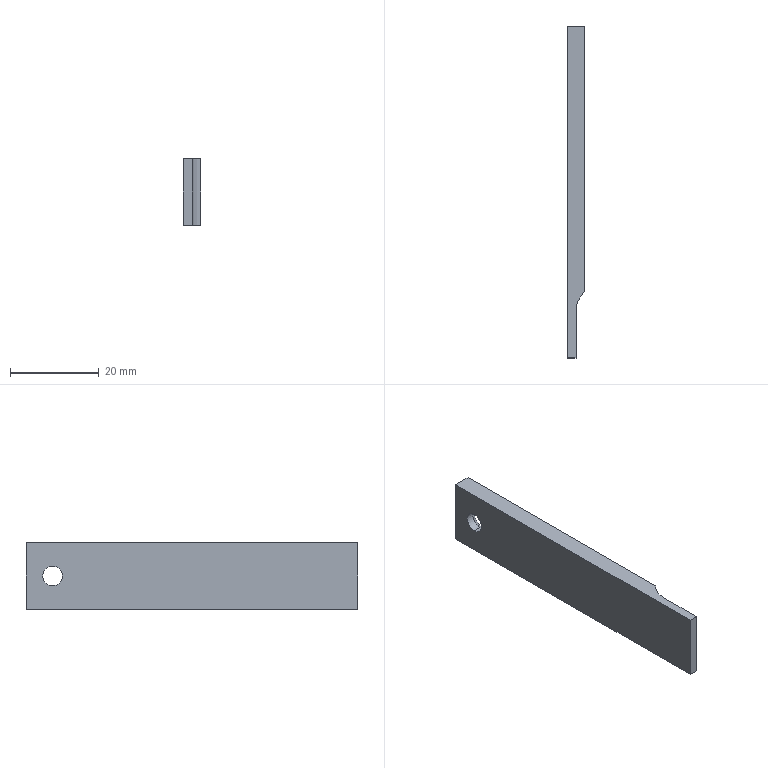Part | NX | features BREP 1 | 1 solid | 12 faces | box 4 x 75 x 15 mm | volume 3981 mm3 | plane 7 | cylinder 3 | cone 2 | commonest cylinder face diameters 4.5 x2 12 x1
STEP:
#1=CARTESIAN_POINT('',(-377.307,34.363,9.75));
#2=VERTEX_POINT('',#1);
#3=CARTESIAN_POINT('',(-377.307,34.363,5.25));
#4=VERTEX_POINT('',#3);
#5=CARTESIAN_POINT('',(-377.307,34.363,7.5));
#6=DIRECTION('',(1.,0.,0.));
#7=DIRECTION('',(0.,0.,-1.));
#8=AXIS2_PLACEMENT_3D('',#5,#6,#7);
#9=CIRCLE('',#8,2.25);
#10=EDGE_CURVE('',#2,#4,#9,.T.);
#11=ORIENTED_EDGE('',*,*,#10,.F.);
#12=CARTESIAN_POINT('',(-375.077,34.363,11.98));
#13=VERTEX_POINT('',#12);
#14=CARTESIAN_POINT('',(-375.077,34.363,11.98));
#15=DIRECTION('',(0.7071,0.,0.7071));
#16=VECTOR('',#15,1000.);
#17=LINE('',#14,#16);
#18=EDGE_CURVE('',#2,#13,#17,.T.);
#19=ORIENTED_EDGE('',*,*,#18,.T.);
#20=CARTESIAN_POINT('',(-375.077,34.363,3.02));
#21=VERTEX_POINT('',#20);
#22=CARTESIAN_POINT('',(-375.077,34.363,7.5));
#23=DIRECTION('',(1.,0.,0.));
#24=DIRECTION('',(0.,0.,-1.));
#25=AXIS2_PLACEMENT_3D('',#22,#23,#24);
#26=CIRCLE('',#25,4.48);
#27=EDGE_CURVE('',#13,#21,#26,.T.);
#28=ORIENTED_EDGE('',*,*,#27,.T.);
#29=CARTESIAN_POINT('',(-375.077,34.363,3.02));
#30=DIRECTION('',(0.7071,0.,-0.7071));
#31=VECTOR('',#30,1000.);
#32=LINE('',#29,#31);
#33=EDGE_CURVE('',#4,#21,#32,.T.);
#34=ORIENTED_EDGE('',*,*,#33,.F.);
#35=EDGE_LOOP('',(#11,#19,#28,#34));
#36=FACE_BOUND('',#35,.T.);
#37=CARTESIAN_POINT('',(-375.077,34.363,7.5));
#38=DIRECTION('',(1.,0.,0.));
#39=DIRECTION('',(0.,0.,-1.));
#40=AXIS2_PLACEMENT_3D('',#37,#38,#39);
#41=CONICAL_SURFACE('',#40,4.48,0.7854);
#42=ADVANCED_FACE('',(#36),#41,.F.);
#43=CARTESIAN_POINT('',(-379.077,34.363,9.75));
#44=VERTEX_POINT('',#43);
#45=CARTESIAN_POINT('',(-379.077,34.363,5.25));
#46=VERTEX_POINT('',#45);
#47=CARTESIAN_POINT('',(-379.077,34.363,7.5));
#48=DIRECTION('',(1.,0.,0.));
#49=DIRECTION('',(0.,0.,-1.));
#50=AXIS2_PLACEMENT_3D('',#47,#48,#49);
#51=CIRCLE('',#50,2.25);
#52=EDGE_CURVE('',#44,#46,#51,.T.);
#53=ORIENTED_EDGE('',*,*,#52,.F.);
#54=CARTESIAN_POINT('',(-375.077,34.363,9.75));
#55=DIRECTION('',(1.,0.,0.));
#56=VECTOR('',#55,1000.);
#57=LINE('',#54,#56);
#58=EDGE_CURVE('',#44,#2,#57,.T.);
#59=ORIENTED_EDGE('',*,*,#58,.T.);
#60=ORIENTED_EDGE('',*,*,#10,.T.);
#61=CARTESIAN_POINT('',(-375.077,34.363,5.25));
#62=DIRECTION('',(1.,0.,0.));
#63=VECTOR('',#62,1000.);
#64=LINE('',#61,#63);
#65=EDGE_CURVE('',#46,#4,#64,.T.);
#66=ORIENTED_EDGE('',*,*,#65,.F.);
#67=EDGE_LOOP('',(#53,#59,#60,#66));
#68=FACE_BOUND('',#67,.T.);
#69=CARTESIAN_POINT('',(-375.077,34.363,7.5));
#70=DIRECTION('',(1.,0.,0.));
#71=DIRECTION('',(0.,0.,-1.));
#72=AXIS2_PLACEMENT_3D('',#69,#70,#71);
#73=CYLINDRICAL_SURFACE('',#72,2.25);
#74=ADVANCED_FACE('',(#68),#73,.F.);
#75=CARTESIAN_POINT('',(-379.077,40.363,0.));
#76=VERTEX_POINT('',#75);
#77=CARTESIAN_POINT('',(-379.077,-34.637,0.));
#78=VERTEX_POINT('',#77);
#79=CARTESIAN_POINT('',(-379.077,40.363,0.));
#80=DIRECTION('',(0.,-1.,0.));
#81=VECTOR('',#80,1000.);
#82=LINE('',#79,#81);
#83=EDGE_CURVE('',#76,#78,#82,.T.);
#84=ORIENTED_EDGE('',*,*,#83,.T.);
#85=CARTESIAN_POINT('',(-379.077,-34.637,15.));
#86=VERTEX_POINT('',#85);
#87=CARTESIAN_POINT('',(-379.077,-34.637,15.));
#88=DIRECTION('',(0.,0.,-1.));
#89=VECTOR('',#88,1000.);
#90=LINE('',#87,#89);
#91=EDGE_CURVE('',#86,#78,#90,.T.);
#92=ORIENTED_EDGE('',*,*,#91,.F.);
#93=CARTESIAN_POINT('',(-379.077,40.363,15.));
#94=VERTEX_POINT('',#93);
#95=CARTESIAN_POINT('',(-379.077,40.363,15.));
#96=DIRECTION('',(0.,-1.,0.));
#97=VECTOR('',#96,1000.);
#98=LINE('',#95,#97);
#99=EDGE_CURVE('',#94,#86,#98,.T.);
#100=ORIENTED_EDGE('',*,*,#99,.F.);
#101=CARTESIAN_POINT('',(-379.077,40.363,15.));
#102=DIRECTION('',(0.,0.,-1.));
#103=VECTOR('',#102,1000.);
#104=LINE('',#101,#103);
#105=EDGE_CURVE('',#94,#76,#104,.T.);
#106=ORIENTED_EDGE('',*,*,#105,.T.);
#107=EDGE_LOOP('',(#84,#92,#100,#106));
#108=FACE_BOUND('',#107,.T.);
#109=CARTESIAN_POINT('',(-379.077,34.363,7.5));
#110=DIRECTION('',(1.,0.,0.));
#111=DIRECTION('',(0.,0.,-1.));
#112=AXIS2_PLACEMENT_3D('',#109,#110,#111);
#113=CIRCLE('',#112,2.25);
#114=EDGE_CURVE('',#46,#44,#113,.T.);
#115=ORIENTED_EDGE('',*,*,#114,.T.);
#116=ORIENTED_EDGE('',*,*,#52,.T.);
#117=EDGE_LOOP('',(#115,#116));
#118=FACE_BOUND('',#117,.T.);
#119=CARTESIAN_POINT('',(-379.077,40.363,15.));
#120=DIRECTION('',(1.,0.,0.));
#121=DIRECTION('',(0.,1.,0.));
#122=AXIS2_PLACEMENT_3D('',#119,#120,#121);
#123=PLANE('',#122);
#124=ADVANCED_FACE('',(#108,#118),#123,.F.);
#125=CARTESIAN_POINT('',(-377.077,-34.637,0.));
#126=VERTEX_POINT('',#125);
#127=CARTESIAN_POINT('',(-379.077,-34.637,0.));
#128=DIRECTION('',(1.,0.,0.));
#129=VECTOR('',#128,1000.);
#130=LINE('',#127,#129);
#131=EDGE_CURVE('',#78,#126,#130,.T.);
#132=ORIENTED_EDGE('',*,*,#131,.T.);
#133=CARTESIAN_POINT('',(-377.077,-34.637,15.));
#134=VERTEX_POINT('',#133);
#135=CARTESIAN_POINT('',(-377.077,-34.637,0.));
#136=DIRECTION('',(0.,0.,1.));
#137=VECTOR('',#136,1000.);
#138=LINE('',#135,#137);
#139=EDGE_CURVE('',#126,#134,#138,.T.);
#140=ORIENTED_EDGE('',*,*,#139,.T.);
#141=CARTESIAN_POINT('',(-379.077,-34.637,15.));
#142=DIRECTION('',(1.,0.,0.));
#143=VECTOR('',#142,1000.);
#144=LINE('',#141,#143);
#145=EDGE_CURVE('',#86,#134,#144,.T.);
#146=ORIENTED_EDGE('',*,*,#145,.F.);
#147=ORIENTED_EDGE('',*,*,#91,.T.);
#148=EDGE_LOOP('',(#132,#140,#146,#147));
#149=FACE_BOUND('',#148,.T.);
#150=CARTESIAN_POINT('',(-379.077,-34.637,15.));
#151=DIRECTION('',(0.,1.,0.));
#152=DIRECTION('',(1.,0.,0.));
#153=AXIS2_PLACEMENT_3D('',#150,#151,#152);
#154=PLANE('',#153);
#155=ADVANCED_FACE('',(#149),#154,.F.);
#156=CARTESIAN_POINT('',(-375.077,-19.637,15.));
#157=VERTEX_POINT('',#156);
#158=CARTESIAN_POINT('',(-375.077,40.363,15.));
#159=VERTEX_POINT('',#158);
#160=CARTESIAN_POINT('',(-375.077,40.363,15.));
#161=DIRECTION('',(0.,1.,0.));
#162=VECTOR('',#161,1000.);
#163=LINE('',#160,#162);
#164=EDGE_CURVE('',#157,#159,#163,.T.);
#165=ORIENTED_EDGE('',*,*,#164,.F.);
#166=CARTESIAN_POINT('',(-375.077,-19.637,0.));
#167=VERTEX_POINT('',#166);
#168=CARTESIAN_POINT('',(-375.077,-19.637,0.));
#169=DIRECTION('',(0.,0.,1.));
#170=VECTOR('',#169,1000.);
#171=LINE('',#168,#170);
#172=EDGE_CURVE('',#167,#157,#171,.T.);
#173=ORIENTED_EDGE('',*,*,#172,.F.);
#174=CARTESIAN_POINT('',(-375.077,40.363,0.));
#175=VERTEX_POINT('',#174);
#176=CARTESIAN_POINT('',(-375.077,40.363,0.));
#177=DIRECTION('',(0.,1.,0.));
#178=VECTOR('',#177,1000.);
#179=LINE('',#176,#178);
#180=EDGE_CURVE('',#167,#175,#179,.T.);
#181=ORIENTED_EDGE('',*,*,#180,.T.);
#182=CARTESIAN_POINT('',(-375.077,40.363,15.));
#183=DIRECTION('',(0.,0.,-1.));
#184=VECTOR('',#183,1000.);
#185=LINE('',#182,#184);
#186=EDGE_CURVE('',#159,#175,#185,.T.);
#187=ORIENTED_EDGE('',*,*,#186,.F.);
#188=EDGE_LOOP('',(#165,#173,#181,#187));
#189=FACE_BOUND('',#188,.T.);
#190=CARTESIAN_POINT('',(-375.077,34.363,7.5));
#191=DIRECTION('',(1.,0.,0.));
#192=DIRECTION('',(0.,0.,-1.));
#193=AXIS2_PLACEMENT_3D('',#190,#191,#192);
#194=CIRCLE('',#193,4.48);
#195=EDGE_CURVE('',#21,#13,#194,.T.);
#196=ORIENTED_EDGE('',*,*,#195,.F.);
#197=ORIENTED_EDGE('',*,*,#27,.F.);
#198=EDGE_LOOP('',(#196,#197));
#199=FACE_BOUND('',#198,.T.);
#200=CARTESIAN_POINT('',(-375.077,40.363,15.));
#201=DIRECTION('',(-1.,0.,0.));
#202=DIRECTION('',(0.,0.,1.));
#203=AXIS2_PLACEMENT_3D('',#200,#201,#202);
#204=PLANE('',#203);
#205=ADVANCED_FACE('',(#189,#199),#204,.F.);
#206=CARTESIAN_POINT('',(-379.077,40.363,0.));
#207=DIRECTION('',(-1.,0.,0.));
#208=VECTOR('',#207,1000.);
#209=LINE('',#206,#208);
#210=EDGE_CURVE('',#175,#76,#209,.T.);
#211=ORIENTED_EDGE('',*,*,#210,.T.);
#212=ORIENTED_EDGE('',*,*,#105,.F.);
#213=CARTESIAN_POINT('',(-379.077,40.363,15.));
#214=DIRECTION('',(-1.,0.,0.));
#215=VECTOR('',#214,1000.);
#216=LINE('',#213,#215);
#217=EDGE_CURVE('',#159,#94,#216,.T.);
#218=ORIENTED_EDGE('',*,*,#217,.F.);
#219=ORIENTED_EDGE('',*,*,#186,.T.);
#220=EDGE_LOOP('',(#211,#212,#218,#219));
#221=FACE_BOUND('',#220,.T.);
#222=CARTESIAN_POINT('',(-379.077,40.363,15.));
#223=DIRECTION('',(0.,-1.,0.));
#224=DIRECTION('',(0.,0.,-1.));
#225=AXIS2_PLACEMENT_3D('',#222,#223,#224);
#226=PLANE('',#225);
#227=ADVANCED_FACE('',(#221),#226,.F.);
#228=CARTESIAN_POINT('',(-377.077,-24.109,15.));
#229=VERTEX_POINT('',#228);
#230=CARTESIAN_POINT('',(-377.077,-34.637,15.));
#231=DIRECTION('',(0.,-1.,0.));
#232=VECTOR('',#231,1000.);
#233=LINE('',#230,#232);
#234=EDGE_CURVE('',#229,#134,#233,.T.);
#235=ORIENTED_EDGE('',*,*,#234,.F.);
#236=CARTESIAN_POINT('',(-371.077,-24.109,15.));
#237=DIRECTION('',(0.,0.,-1.));
#238=DIRECTION('',(1.,0.,0.));
#239=AXIS2_PLACEMENT_3D('',#236,#237,#238);
#240=CIRCLE('',#239,6.);
#241=EDGE_CURVE('',#229,#157,#240,.T.);
#242=ORIENTED_EDGE('',*,*,#241,.T.);
#243=ORIENTED_EDGE('',*,*,#164,.T.);
#244=ORIENTED_EDGE('',*,*,#217,.T.);
#245=ORIENTED_EDGE('',*,*,#99,.T.);
#246=ORIENTED_EDGE('',*,*,#145,.T.);
#247=EDGE_LOOP('',(#235,#242,#243,#244,#245,#246));
#248=FACE_BOUND('',#247,.T.);
#249=CARTESIAN_POINT('',(-379.077,-34.637,15.));
#250=DIRECTION('',(0.,0.,1.));
#251=DIRECTION('',(1.,0.,0.));
#252=AXIS2_PLACEMENT_3D('',#249,#250,#251);
#253=PLANE('',#252);
#254=ADVANCED_FACE('',(#248),#253,.T.);
#255=ORIENTED_EDGE('',*,*,#180,.F.);
#256=CARTESIAN_POINT('',(-377.077,-24.109,0.));
#257=VERTEX_POINT('',#256);
#258=CARTESIAN_POINT('',(-371.077,-24.109,0.));
#259=DIRECTION('',(0.,0.,1.));
#260=DIRECTION('',(1.,0.,0.));
#261=AXIS2_PLACEMENT_3D('',#258,#259,#260);
#262=CIRCLE('',#261,6.);
#263=EDGE_CURVE('',#167,#257,#262,.T.);
#264=ORIENTED_EDGE('',*,*,#263,.T.);
#265=CARTESIAN_POINT('',(-377.077,-34.637,0.));
#266=DIRECTION('',(0.,-1.,0.));
#267=VECTOR('',#266,1000.);
#268=LINE('',#265,#267);
#269=EDGE_CURVE('',#257,#126,#268,.T.);
#270=ORIENTED_EDGE('',*,*,#269,.T.);
#271=ORIENTED_EDGE('',*,*,#131,.F.);
#272=ORIENTED_EDGE('',*,*,#83,.F.);
#273=ORIENTED_EDGE('',*,*,#210,.F.);
#274=EDGE_LOOP('',(#255,#264,#270,#271,#272,#273));
#275=FACE_BOUND('',#274,.T.);
#276=CARTESIAN_POINT('',(-379.077,-34.637,0.));
#277=DIRECTION('',(0.,0.,1.));
#278=DIRECTION('',(1.,0.,0.));
#279=AXIS2_PLACEMENT_3D('',#276,#277,#278);
#280=PLANE('',#279);
#281=ADVANCED_FACE('',(#275),#280,.F.);
#282=ORIENTED_EDGE('',*,*,#269,.F.);
#283=CARTESIAN_POINT('',(-377.077,-24.109,0.));
#284=DIRECTION('',(0.,0.,1.));
#285=VECTOR('',#284,1000.);
#286=LINE('',#283,#285);
#287=EDGE_CURVE('',#257,#229,#286,.T.);
#288=ORIENTED_EDGE('',*,*,#287,.T.);
#289=ORIENTED_EDGE('',*,*,#234,.T.);
#290=ORIENTED_EDGE('',*,*,#139,.F.);
#291=EDGE_LOOP('',(#282,#288,#289,#290));
#292=FACE_BOUND('',#291,.T.);
#293=CARTESIAN_POINT('',(-377.077,-34.637,0.));
#294=DIRECTION('',(-1.,0.,0.));
#295=DIRECTION('',(0.,0.,1.));
#296=AXIS2_PLACEMENT_3D('',#293,#294,#295);
#297=PLANE('',#296);
#298=ADVANCED_FACE('',(#292),#297,.F.);
#299=ORIENTED_EDGE('',*,*,#263,.F.);
#300=ORIENTED_EDGE('',*,*,#172,.T.);
#301=ORIENTED_EDGE('',*,*,#241,.F.);
#302=ORIENTED_EDGE('',*,*,#287,.F.);
#303=EDGE_LOOP('',(#299,#300,#301,#302));
#304=FACE_BOUND('',#303,.T.);
#305=CARTESIAN_POINT('',(-371.077,-24.109,0.));
#306=DIRECTION('',(0.,0.,1.));
#307=DIRECTION('',(1.,0.,0.));
#308=AXIS2_PLACEMENT_3D('',#305,#306,#307);
#309=CYLINDRICAL_SURFACE('',#308,6.);
#310=ADVANCED_FACE('',(#304),#309,.F.);
#311=ORIENTED_EDGE('',*,*,#58,.F.);
#312=ORIENTED_EDGE('',*,*,#114,.F.);
#313=ORIENTED_EDGE('',*,*,#65,.T.);
#314=CARTESIAN_POINT('',(-377.307,34.363,7.5));
#315=DIRECTION('',(1.,0.,0.));
#316=DIRECTION('',(0.,0.,-1.));
#317=AXIS2_PLACEMENT_3D('',#314,#315,#316);
#318=CIRCLE('',#317,2.25);
#319=EDGE_CURVE('',#4,#2,#318,.T.);
#320=ORIENTED_EDGE('',*,*,#319,.T.);
#321=EDGE_LOOP('',(#311,#312,#313,#320));
#322=FACE_BOUND('',#321,.T.);
#323=CARTESIAN_POINT('',(-375.077,34.363,7.5));
#324=DIRECTION('',(1.,0.,0.));
#325=DIRECTION('',(0.,0.,-1.));
#326=AXIS2_PLACEMENT_3D('',#323,#324,#325);
#327=CYLINDRICAL_SURFACE('',#326,2.25);
#328=ADVANCED_FACE('',(#322),#327,.F.);
#329=ORIENTED_EDGE('',*,*,#18,.F.);
#330=ORIENTED_EDGE('',*,*,#319,.F.);
#331=ORIENTED_EDGE('',*,*,#33,.T.);
#332=ORIENTED_EDGE('',*,*,#195,.T.);
#333=EDGE_LOOP('',(#329,#330,#331,#332));
#334=FACE_BOUND('',#333,.T.);
#335=CARTESIAN_POINT('',(-375.077,34.363,7.5));
#336=DIRECTION('',(1.,0.,0.));
#337=DIRECTION('',(0.,0.,-1.));
#338=AXIS2_PLACEMENT_3D('',#335,#336,#337);
#339=CONICAL_SURFACE('',#338,4.48,0.7854);
#340=ADVANCED_FACE('',(#334),#339,.F.);
#341=CLOSED_SHELL('',(#42,#74,#124,#155,#205,#227,#254,#281,#298,#310,#328,#340));
#342=MANIFOLD_SOLID_BREP('',#341);
#343=(LENGTH_UNIT()NAMED_UNIT(*)SI_UNIT(.MILLI.,.METRE.));
#344=UNCERTAINTY_MEASURE_WITH_UNIT(LENGTH_MEASURE(0.00001),#343,'','');
#345=(NAMED_UNIT(*)PLANE_ANGLE_UNIT()SI_UNIT($,.RADIAN.));
#346=(NAMED_UNIT(*)SI_UNIT($,.STERADIAN.)SOLID_ANGLE_UNIT());
#347=(GEOMETRIC_REPRESENTATION_CONTEXT(3)GLOBAL_UNCERTAINTY_ASSIGNED_CONTEXT((#344))GLOBAL_UNIT_ASSIGNED_CONTEXT((#343,#345,#346))REPRESENTATION_CONTEXT('',''));
#348=ADVANCED_BREP_SHAPE_REPRESENTATION('',(#342),#347);